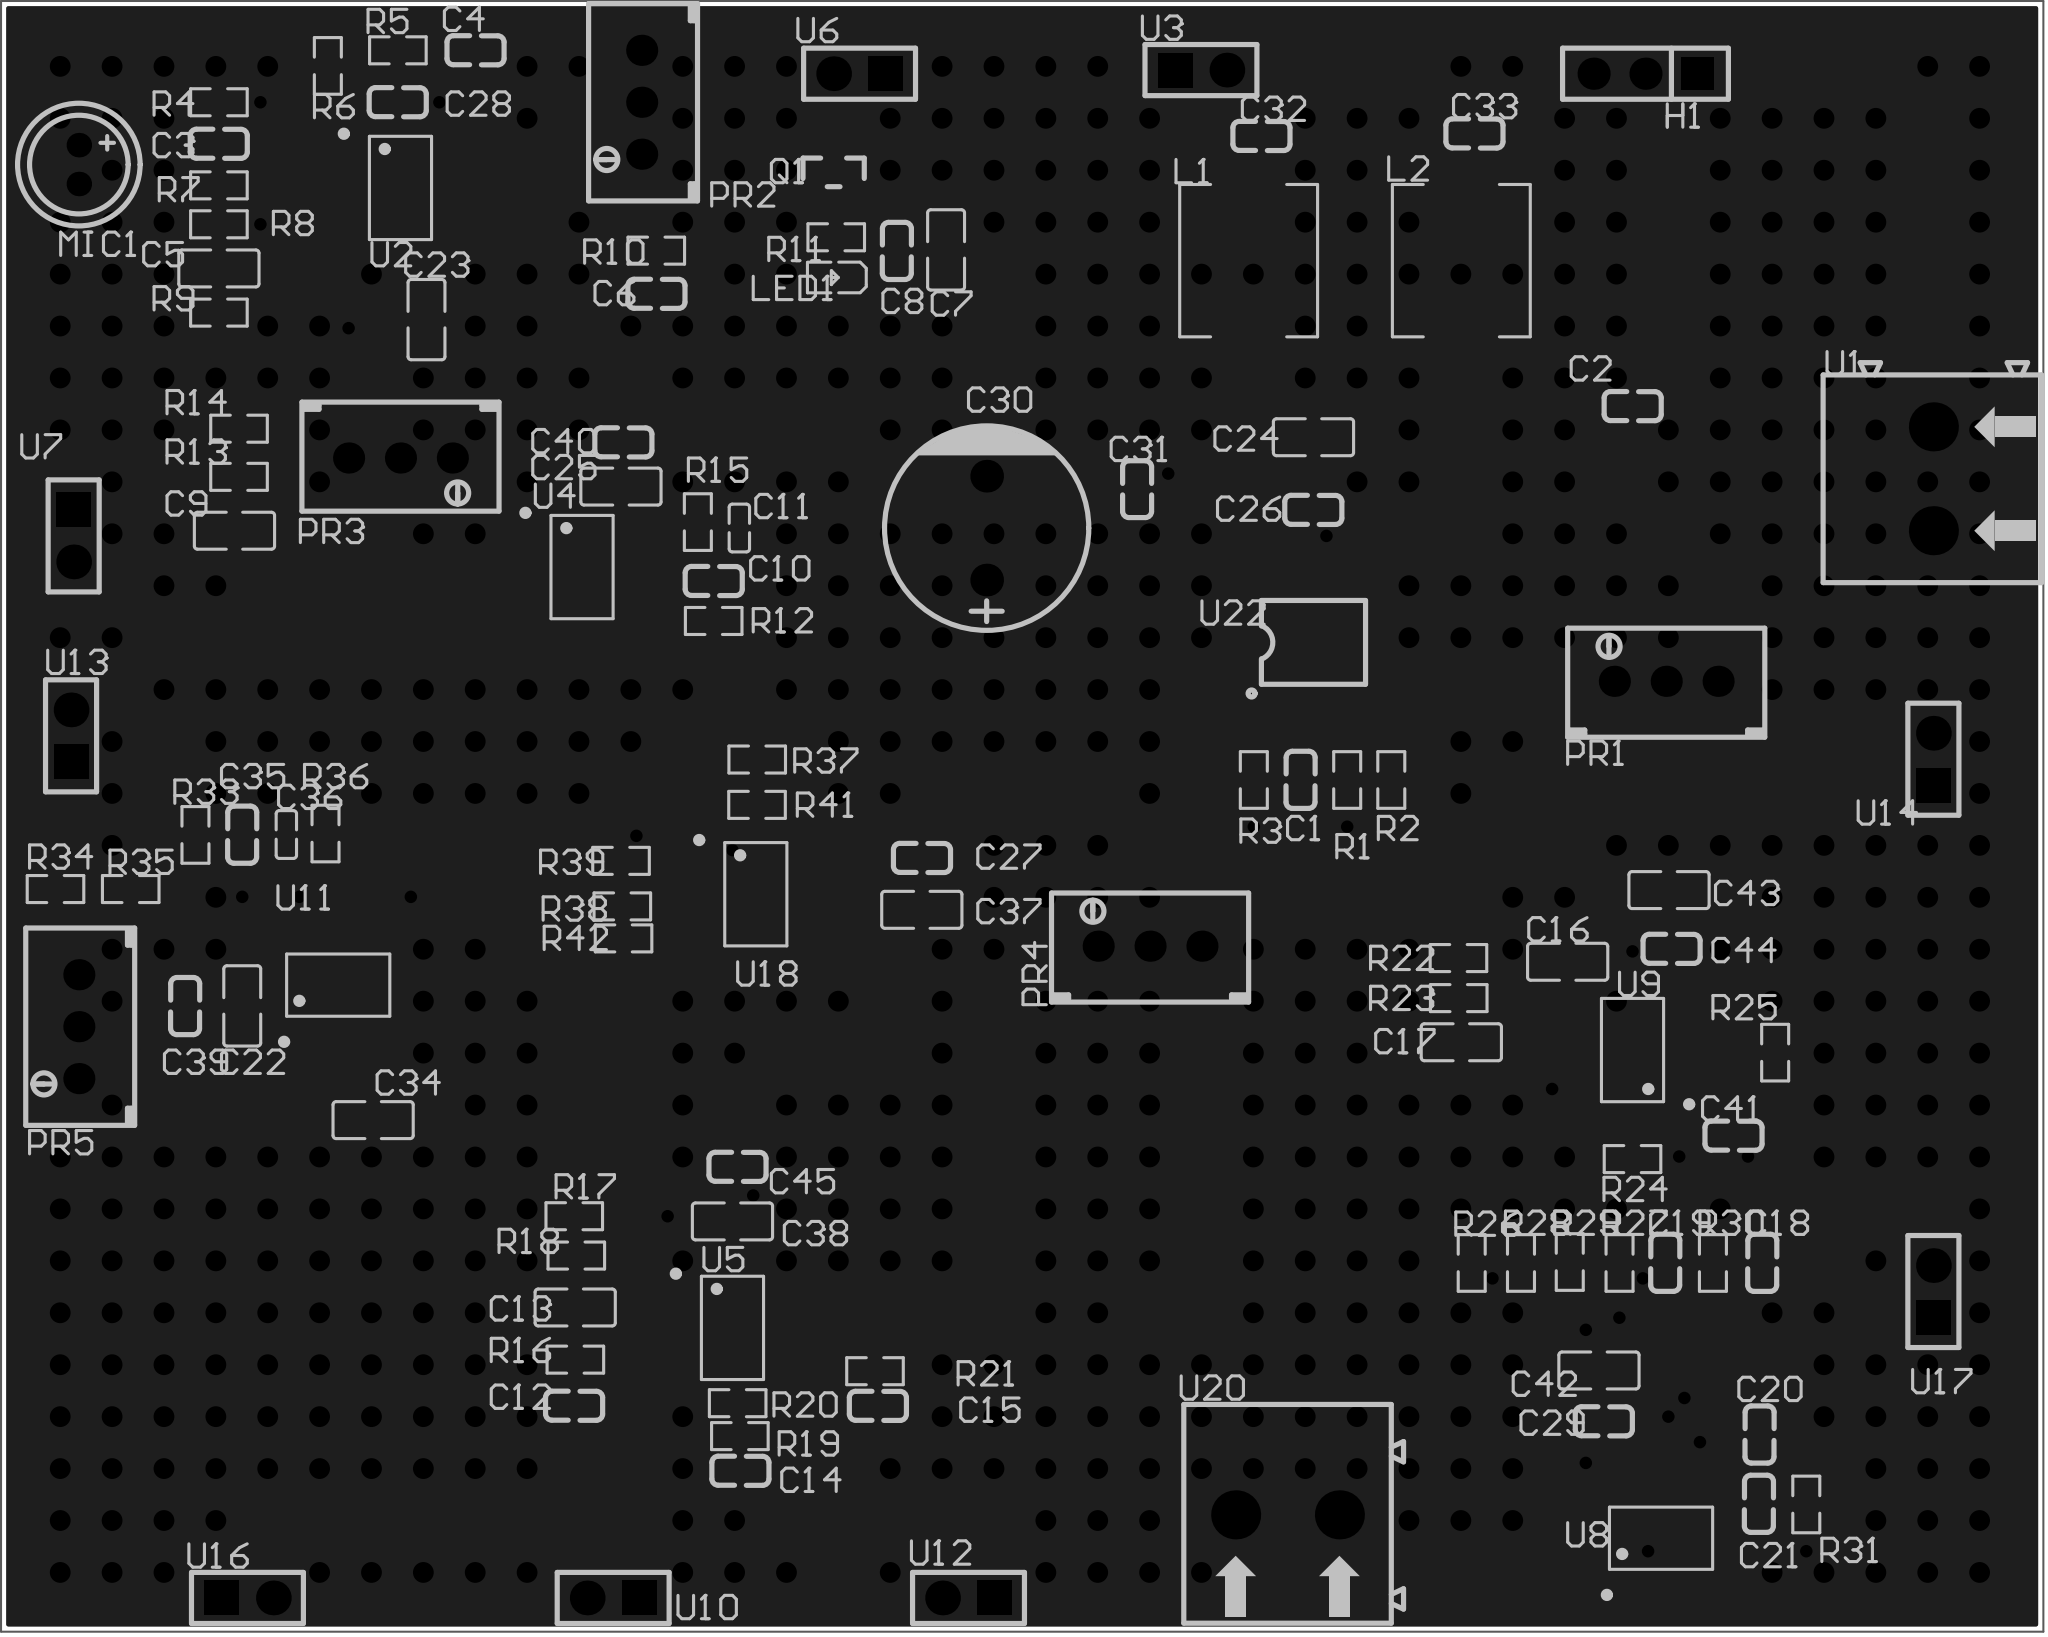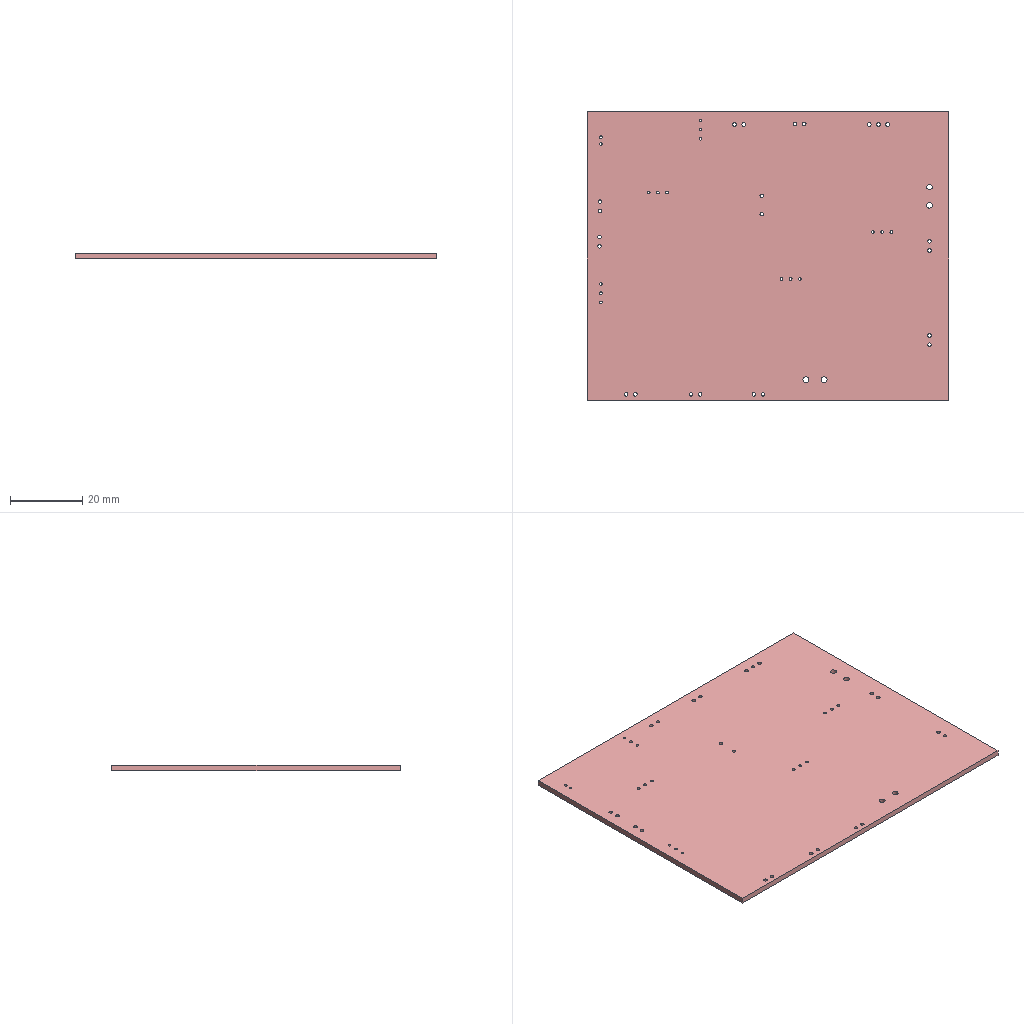Circuit board layout | Altium Designer | box 100 x 79.8 x 1.6 mm
Layer stack:
# Altium Designer layer stack of  (unit mm; dielectric type: 0 none, 1 core, 2 prepreg, 3 surface material)
index,name,kind,layer,copper_thickness_mm,dielectric_type,dielectric_thickness_mm,dielectric_material,dielectric_constant
0,Top Paste Mask Layer,other,,,,,,
1,Top Silkscreen Layer,other,,,,,,
2,Top Solder Mask Layer,dielectric,,,3,0.01,,3.3
3,Top Layer,copper,Top Layer,0.035,,,,
4,Dielectric1,dielectric,,,3,1.51,FR4,4.5
5,Bottom Layer,copper,Bottom Layer,0.035,,,,
6,Bottom Solder Mask Layer,dielectric,,,3,0.01,,3.3
7,Bottom Silkscreen Layer,other,,,,,,
8,Bottom Paste Mask Layer,other,,,,,,
# drill layer pairs: low layer,high layer
drill_pair,Top Layer,Bottom Layer
Part placement:
Designator,Comment,Layer,Footprint,Center-X(mm),Center-Y(mm),Rotation
C1,1uF,TopLayer,C0603,158.369,131.318,270
C2,470nF,TopLayer,C0603,174.625,149.606,180
C3,1uF,TopLayer,C0603,105.41,162.433,0
C4,1uF,TopLayer,C0603,117.983,167.005,0
C5,100nF,TopLayer,C0805,105.41,156.337,0
C6,1uF,TopLayer,C0603,126.825,155.099,180
C7,100nF,TopLayer,C0805,141.015,157.244,270
C8,1uF,TopLayer,C0603,138.602,157.186,270
C9,100nF,TopLayer,C0805,106.172,143.51,0
C10,1uF,TopLayer,C0603,129.63,141.054,180
C11,3.3pF,TopLayer,C0402,130.893,143.642,270
C12,1uF,TopLayer,C0603,122.809,100.711,0
C13,100nF,TopLayer,C0805,122.855,105.519,180
C14,1uF,TopLayer,C0603,130.937,97.536,180
C15,1uF,TopLayer,C0603,137.668,100.711,180
C16,2.2nF,TopLayer,C0805,171.45,122.428,180
C17,2.2nF,TopLayer,C0805,166.243,118.491,0
C18,27nF,TopLayer,C0603,180.975,107.696,270
C19,27nF,TopLayer,C0603,176.231,107.713,90
C20,68nF,TopLayer,C0603,180.848,99.314,90
C21,68nF,TopLayer,C0603,180.817,95.926,90
C22,100nF,TopLayer,C0805,106.553,120.269,90
C23,100nF,TopLayer,C0805,115.574,153.834,90
C24,100nF,TopLayer,C0805,159.004,148.082,0
C25,100nF,TopLayer,C0805,125.095,145.669,0
C26,10uF,TopLayer,C0603,159.004,144.526,0
C27,10uF,TopLayer,C0603,139.827,127.508,180
C28,10uF,TopLayer,C0603,114.173,164.465,0
C29,10uF,TopLayer,C0603,173.228,99.949,0
C30,470uF,TopLayer,CAP-TH_BD10.0-P5.00-D1.0-FD,143.002,143.637,90
C31,1uF,TopLayer,C0603,150.368,145.542,90
C32,1uF,TopLayer,C0603,156.464,162.814,0
C33,1uF,TopLayer,C0603,166.878,162.941,180
C34,100nF,TopLayer,C0805,112.96,114.683,180
C35,1uF,TopLayer,C0603,106.553,128.651,90
C36,3.3pF,TopLayer,C0402,108.712,128.651,90
C37,100nF,TopLayer,C0805,139.827,124.968,180
C38,100nF,TopLayer,C0805,130.556,109.728,0
C39,10uF,TopLayer,C0603,103.759,120.269,90
C40,10uF,TopLayer,C0603,125.222,147.828,0
C41,6.8nF,TopLayer,C0603,179.578,113.919,0
H1,PM254V-11-03-H85,TopLayer,HDR-TH_3P-P2.54-V-F,175.26,165.862,180
L1,33uH,TopLayer,IND-SMD_L7.3-W6.6,155.829,156.718,270
L2,33uH,TopLayer,IND-SMD_L7.3-W6.6,166.243,156.718,270
LED1,NCD0603G1,TopLayer,LED0603-RD,135.617,155.9,180
MIC1,GMI6050P-36db,TopLayer,MIC-TH_BD6.0-P1.90-D0.4-L-FD_GMI6050P-2CXXDB,98.552,161.417,270
PR1,500kΩ,TopLayer,RES-ADJ-TH_3296W,176.276,136.144,90
PR2,10kΩ,TopLayer,RES-ADJ-TH_3296W,126.111,164.465,180
PR3,10kΩ,TopLayer,RES-ADJ-TH_3296W,114.3,147.066,270
PR4,10kΩ,TopLayer,RES-ADJ-TH_3296W,151.003,123.19,90
PR5,10kΩ,TopLayer,RES-ADJ-TH_3296W,98.552,119.253,180
Q1,AO3401A,TopLayer,SOT-23_L2.9-W1.3-P1.90-LS2.4-BR,135.509,161.036,270
R1,10kΩ,TopLayer,R0603,160.655,131.318,270
R2,10kΩ,TopLayer,R0603,162.814,131.318,90
R3,10kΩ,TopLayer,R0603,156.083,131.318,270
R4,10kΩ,TopLayer,R0603,105.41,164.465,0
R5,0603WAF1001T5E,TopLayer,R0603,114.173,167.005,0
R6,20kΩ,TopLayer,R0603,110.744,166.243,90
R7,0603WAF7502T5E,TopLayer,R0603,105.41,160.401,0
R8,47kΩ,TopLayer,R0603,105.41,158.496,0
R9,47kΩ,TopLayer,R0603,105.41,154.178,180
R10,0603WAF1001T5E,TopLayer,R0603,126.825,157.208,180
R11,10kΩ,TopLayer,R0603,135.636,157.861,180
R12,100kΩ,TopLayer,R0603,129.636,139.095,180
R13,0Ω,TopLayer,R0603,106.395,146.145,0
R14,0603WAF1001T5E,TopLayer,R0603,106.395,148.499,0
R15,1MΩ,TopLayer,R0603,128.861,143.931,90
R16,0603WAF7502T5E,TopLayer,R0603,122.863,102.969,180
R17,47kΩ,TopLayer,R0603,122.809,109.982,0
R18,47kΩ,TopLayer,R0603,122.909,108.059,180
R19,0603WAF1001T5E,TopLayer,R0603,130.918,99.228,0
R20,20kΩ,TopLayer,R0603,130.81,100.838,0
R21,0603WAF1001T5E,TopLayer,R0603,137.535,102.403,0
R22,20kΩ,TopLayer,R0603,166.103,122.608,0
R23,20kΩ,TopLayer,R0603,166.116,120.65,180
R24,20kΩ,TopLayer,R0603,174.625,112.776,180
R25,20kΩ,TopLayer,R0603,181.61,117.983,270
R26,20kΩ,TopLayer,R0603,166.751,107.696,90
R27,0603WAF1001T5E,TopLayer,R0603,173.99,107.696,270
R28,11kΩ,TopLayer,R0603,169.164,107.696,90
R29,20kΩ,TopLayer,R0603,171.552,107.743,270
R30,16kΩ,TopLayer,R0603,178.562,107.696,90
R31,0603WAF3001T5E,TopLayer,R0603,183.134,95.885,90
R33,100kΩ,TopLayer,R0603,104.262,128.632,90
R34,0Ω,TopLayer,R0603,97.409,125.984,180
R35,0603WAF1001T5E,TopLayer,R0603,101.092,125.984,0
R36,1MΩ,TopLayer,R0603,110.63,128.701,270
R37,10kΩ,TopLayer,R0603,131.767,132.319,0
R38,10kΩ,TopLayer,R0603,125.163,125.135,0
R39,10kΩ,TopLayer,R0603,125.099,127.363,0
R41,10kΩ,TopLayer,R0603,131.758,130.102,0
R42,10kΩ,TopLayer,R0603,125.222,123.571,0
U1,KF128-5.08-2P-AA,TopLayer,CONN-TH_P5.08_KF128-5.08-2P,189.357,146.05,90
U2,NE5532DR,TopLayer,SOIC-8_L4.9-W3.9-P1.27-LS6.0-BL,114.3,160.274,270
U3,ZX-PM2.54-1-2PY,TopLayer,HDR-TH_2P-P2.54-V-F,153.494,166.039,0
U4,NE5532DR,TopLayer,SOIC-8_L4.9-W3.9-P1.27-LS6.0-BL,123.19,141.732,270
U5,NE5532DR,TopLayer,SOIC-8_L4.9-W3.9-P1.27-LS6.0-BL,130.556,104.521,270
U6,ZX-PM2.54-1-2PY,TopLayer,HDR-TH_2P-P2.54-V-F,136.779,165.862,180
U7,ZX-PM2.54-1-2PY,TopLayer,HDR-TH_2P-P2.54-V-F,98.298,143.256,270
U8,NE5532DR,TopLayer,SOIC-8_L4.9-W3.9-P1.27-LS6.0-BL,176.022,94.234,0
U9,NE5532DR,TopLayer,SOIC-8_L4.9-W3.9-P1.27-LS6.0-BL,174.625,118.11,90
U10,ZX-PM2.54-1-2PY,TopLayer,HDR-TH_2P-P2.54-V-F,124.714,91.313,180
U11,NE5532DR,TopLayer,SOIC-8_L4.9-W3.9-P1.27-LS6.0-BL,111.252,121.285,0
U12,ZX-PM2.54-1-2PY,TopLayer,HDR-TH_2P-P2.54-V-F,142.113,91.313,180
U13,ZX-PM2.54-1-2PY,TopLayer,HDR-TH_2P-P2.54-V-F,98.171,133.477,90
U14,ZX-PM2.54-1-2PY,TopLayer,HDR-TH_2P-P2.54-V-F,189.357,132.334,90
U16,ZX-PM2.54-1-2PY,TopLayer,HDR-TH_2P-P2.54-V-F,106.807,91.313,0
U17,ZX-PM2.54-1-2PY,TopLayer,HDR-TH_2P-P2.54-V-F,189.357,106.299,90
U18,NE5532DR,TopLayer,SOIC-8_L4.9-W3.9-P1.27-LS6.0-BL,131.699,125.73,270
U20,KF128-5.08-2P-AA,TopLayer,CONN-TH_P5.08_KF128-5.08-2P,157.734,95.377,0
U22,XPT8871MS,TopLayer,ESOP-8_L4.9-W3.9-P1.27-LS6.0-BL-EP,159.004,138.049,0
C42,100nF,TopLayer,C0805,172.982,102.438,0
C43,100nF,TopLayer,C0805,176.412,125.933,180
C44,10uF,TopLayer,C0603,176.53,123.063,180
C45,10uF,TopLayer,C0603,130.81,112.395,0
Pad and via stacks:
# Altium Designer via and pad stacks of  (unit mm). Each distinct definition once, with the count of objects using it.
# via: kind,start_layer,end_layer,hole_mm,diameter_mm,mode(0 simple;1 top-mid-bottom;2 full stack),diameter_per_layer,count,example_net
# pad: kind,layer,hole_mm,hole_type(0 round;1 square;2 slot),plating,top_size,top_shape(1 round;2 rect;3 octagon;9 rounded rect),mid_size,bottom_size,mode,footprint,size_per_layer,count,example
pad,Top Layer,0,0,plated,0.8x0.9,2,0.8x0.9,0.8x0.9,0,C0603,,54,C1.2
pad,Top Layer,0,0,plated,1.41x1.35,2,1.41x1.35,1.41x1.35,0,C0805,,30,C5.2
pad,Top Layer,0,0,plated,0.7901x0.54,2,0.7901x0.54,0.7901x0.54,0,C0402,,4,C11.2
pad,Top Layer,0,0,plated,2.423x3.419,2,2.423x3.419,2.423x3.419,0,IND-SMD_L7.3-W6.6,,4,L1.1
pad,Top Layer,0,0,plated,0.8x0.8,2,0.8x0.8,0.8x0.8,0,LED0603-RD,,2,LED1.2
pad,Top Layer,0,0,plated,1x0.8,2,1x0.8,1x0.8,0,SOT-23_L2.9-W1.3-P1.90-LS2.4-BR,,3,Q1.2
pad,Top Layer,0,0,plated,0.8065x0.864,2,0.8065x0.864,0.8065x0.864,0,R0603,,80,R1.2
pad,Top Layer,0,0,plated,0.588x2.045,1,0.588x2.045,0.588x2.045,0,SOIC-8_L4.9-W3.9-P1.27-LS6.0-BL,,56,U2.5
pad,Top Layer,0,0,plated,0.6x1.2,2,0.6x1.2,0.6x1.2,0,ESOP-8_L4.9-W3.9-P1.27-LS6.0-BL-EP,,8,U22.1
pad,Top Layer,0,0,plated,3.3x2.4,2,3.3x2.4,3.3x2.4,0,ESOP-8_L4.9-W3.9-P1.27-LS6.0-BL-EP,,1,U22.9
pad,Multi-Layer,1,0,plated,1.6x1.6,1,1.6x1.6,1.6x1.6,0,CAP-TH_BD10.0-P5.00-D1.0-FD,,2,C30.1
pad,Multi-Layer,1.02,0,plated,1.575x1.575,1,1.575x1.575,1.575x1.575,0,HDR-TH_3P-P2.54-V-F,,2,H1.3
pad,Multi-Layer,1.02,0,plated,1.575x1.575,2,1.575x1.575,1.575x1.575,0,HDR-TH_3P-P2.54-V-F,,1,H1.1
pad,Multi-Layer,0.7,0,plated,1.2x1.2,1,1.2x1.2,1.2x1.2,0,MIC-TH_BD6.0-P1.90-D0.4-L-FD_GMI6050P-2CXXDB,,2,MIC1.1
pad,Multi-Layer,0.762,0,plated,1.524x1.524,1,1.524x1.524,1.524x1.524,0,RES-ADJ-TH_3296W,,15,PR1.2
pad,Multi-Layer,1.6,0,plated,2.4x2.4,1,2.4x2.4,2.4x2.4,0,CONN-TH_P5.08_KF128-5.08-2P,,4,U1.1
pad,Multi-Layer,1,0,plated,1.7x1.7,2,1.7x1.7,1.7x1.7,0,HDR-TH_2P-P2.54-V-F,,9,U3.1
pad,Multi-Layer,1,0,plated,1.7x1.7,1,1.7x1.7,1.7x1.7,0,HDR-TH_2P-P2.54-V-F,,9,U3.2
via,Top Layer,Bottom Layer,0.3048,0.61,0,,29,$1N157
via,Top Layer,Bottom Layer,0.508,1.016,0,,644,GND
Copper pours:
name,layer,net,type(0 solid;1 hatched;2 none)
Top Layer-GND,Top Layer,GND,0
Bottom Layer-GND,Bottom Layer,GND,0
Design rules, without the lines most boards share:
# Altium Designer design rules of  (exported by Altium Designer, unit mm)
# columns: name | kind | enabled | priority | scope1 | scope2 | descriptor | typed fields (field=value)
copperRegion | 20 | enabled | 1 | (InNet('GND')) | All | Polygon Connect Rule(Relief Connect )(Conductor Width=10mil) (Relief Angle=90 Angle) (Entries=4) (Air Gap Width=10mil) ((InNet('GND'))),(All) | connect_style(0=relief,1=direct,2=none)=0 relief_conductor_width=0.254 relief_entries=4